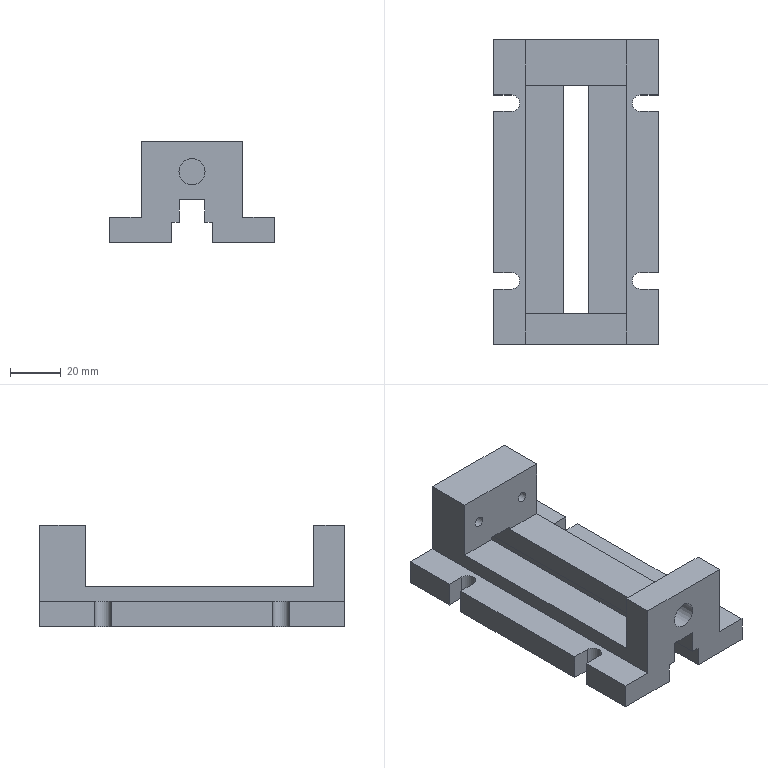Part | NX | features DATUM_CSYS 8, SKETCH 7, EXTRUDE 5, SIMPLE HOLE 5, HOLE PACKAGE 3, SYMBOLIC_THREAD 3 | 1 solid | 47 faces | box 65 x 120 x 40 mm | volume 106229 mm3 | plane 38 | cylinder 9 | commonest cylinder face diameters 6.5 x4 4.2 x2 5 x2 10.3 x1
STEP:
#1=CARTESIAN_POINT('',(-32.5,60.,0.));
#2=VERTEX_POINT('',#1);
#3=CARTESIAN_POINT('',(-32.5,38.25,0.));
#4=VERTEX_POINT('',#3);
#5=CARTESIAN_POINT('',(-32.5,60.,0.));
#6=DIRECTION('',(0.,-1.,0.));
#7=VECTOR('',#6,1000.);
#8=LINE('',#5,#7);
#9=EDGE_CURVE('',#2,#4,#8,.T.);
#10=ORIENTED_EDGE('',*,*,#9,.T.);
#11=CARTESIAN_POINT('',(-32.5,38.25,10.));
#12=VERTEX_POINT('',#11);
#13=CARTESIAN_POINT('',(-32.5,38.25,-1.));
#14=DIRECTION('',(0.,0.,-1.));
#15=VECTOR('',#14,1000.);
#16=LINE('',#13,#15);
#17=EDGE_CURVE('',#4,#12,#16,.F.);
#18=ORIENTED_EDGE('',*,*,#17,.T.);
#19=CARTESIAN_POINT('',(-32.5,60.,10.));
#20=VERTEX_POINT('',#19);
#21=CARTESIAN_POINT('',(-32.5,60.,10.));
#22=DIRECTION('',(0.,-1.,0.));
#23=VECTOR('',#22,1000.);
#24=LINE('',#21,#23);
#25=EDGE_CURVE('',#20,#12,#24,.T.);
#26=ORIENTED_EDGE('',*,*,#25,.F.);
#27=CARTESIAN_POINT('',(-32.5,60.,10.));
#28=DIRECTION('',(0.,0.,-1.));
#29=VECTOR('',#28,1000.);
#30=LINE('',#27,#29);
#31=EDGE_CURVE('',#20,#2,#30,.T.);
#32=ORIENTED_EDGE('',*,*,#31,.T.);
#33=EDGE_LOOP('',(#10,#18,#26,#32));
#34=FACE_BOUND('',#33,.T.);
#35=CARTESIAN_POINT('',(-32.5,60.,10.));
#36=DIRECTION('',(1.,0.,0.));
#37=DIRECTION('',(0.,1.,0.));
#38=AXIS2_PLACEMENT_3D('',#35,#36,#37);
#39=PLANE('',#38);
#40=ADVANCED_FACE('',(#34),#39,.F.);
#41=CARTESIAN_POINT('',(-32.5,31.75,10.));
#42=VERTEX_POINT('',#41);
#43=CARTESIAN_POINT('',(-32.5,-31.75,10.));
#44=VERTEX_POINT('',#43);
#45=CARTESIAN_POINT('',(-32.5,60.,10.));
#46=DIRECTION('',(0.,-1.,0.));
#47=VECTOR('',#46,1000.);
#48=LINE('',#45,#47);
#49=EDGE_CURVE('',#42,#44,#48,.T.);
#50=ORIENTED_EDGE('',*,*,#49,.F.);
#51=CARTESIAN_POINT('',(-32.5,31.75,0.));
#52=VERTEX_POINT('',#51);
#53=CARTESIAN_POINT('',(-32.5,31.75,-1.));
#54=DIRECTION('',(0.,0.,1.));
#55=VECTOR('',#54,1000.);
#56=LINE('',#53,#55);
#57=EDGE_CURVE('',#42,#52,#56,.F.);
#58=ORIENTED_EDGE('',*,*,#57,.T.);
#59=CARTESIAN_POINT('',(-32.5,-31.75,0.));
#60=VERTEX_POINT('',#59);
#61=CARTESIAN_POINT('',(-32.5,60.,0.));
#62=DIRECTION('',(0.,-1.,0.));
#63=VECTOR('',#62,1000.);
#64=LINE('',#61,#63);
#65=EDGE_CURVE('',#52,#60,#64,.T.);
#66=ORIENTED_EDGE('',*,*,#65,.T.);
#67=CARTESIAN_POINT('',(-32.5,-31.75,-1.));
#68=DIRECTION('',(0.,0.,-1.));
#69=VECTOR('',#68,1000.);
#70=LINE('',#67,#69);
#71=EDGE_CURVE('',#60,#44,#70,.F.);
#72=ORIENTED_EDGE('',*,*,#71,.T.);
#73=EDGE_LOOP('',(#50,#58,#66,#72));
#74=FACE_BOUND('',#73,.T.);
#75=CARTESIAN_POINT('',(-32.5,60.,10.));
#76=DIRECTION('',(1.,0.,0.));
#77=DIRECTION('',(0.,1.,0.));
#78=AXIS2_PLACEMENT_3D('',#75,#76,#77);
#79=PLANE('',#78);
#80=ADVANCED_FACE('',(#74),#79,.F.);
#81=CARTESIAN_POINT('',(32.5,-60.,0.));
#82=VERTEX_POINT('',#81);
#83=CARTESIAN_POINT('',(32.5,-38.25,0.));
#84=VERTEX_POINT('',#83);
#85=CARTESIAN_POINT('',(32.5,-60.,0.));
#86=DIRECTION('',(0.,1.,0.));
#87=VECTOR('',#86,1000.);
#88=LINE('',#85,#87);
#89=EDGE_CURVE('',#82,#84,#88,.T.);
#90=ORIENTED_EDGE('',*,*,#89,.T.);
#91=CARTESIAN_POINT('',(32.5,-38.25,10.));
#92=VERTEX_POINT('',#91);
#93=CARTESIAN_POINT('',(32.5,-38.25,-1.));
#94=DIRECTION('',(0.,0.,-1.));
#95=VECTOR('',#94,1000.);
#96=LINE('',#93,#95);
#97=EDGE_CURVE('',#84,#92,#96,.F.);
#98=ORIENTED_EDGE('',*,*,#97,.T.);
#99=CARTESIAN_POINT('',(32.5,-60.,10.));
#100=VERTEX_POINT('',#99);
#101=CARTESIAN_POINT('',(32.5,-60.,10.));
#102=DIRECTION('',(0.,1.,0.));
#103=VECTOR('',#102,1000.);
#104=LINE('',#101,#103);
#105=EDGE_CURVE('',#100,#92,#104,.T.);
#106=ORIENTED_EDGE('',*,*,#105,.F.);
#107=CARTESIAN_POINT('',(32.5,-60.,10.));
#108=DIRECTION('',(0.,0.,-1.));
#109=VECTOR('',#108,1000.);
#110=LINE('',#107,#109);
#111=EDGE_CURVE('',#100,#82,#110,.T.);
#112=ORIENTED_EDGE('',*,*,#111,.T.);
#113=EDGE_LOOP('',(#90,#98,#106,#112));
#114=FACE_BOUND('',#113,.T.);
#115=CARTESIAN_POINT('',(32.5,-60.,10.));
#116=DIRECTION('',(-1.,0.,0.));
#117=DIRECTION('',(0.,-1.,0.));
#118=AXIS2_PLACEMENT_3D('',#115,#116,#117);
#119=PLANE('',#118);
#120=ADVANCED_FACE('',(#114),#119,.F.);
#121=CARTESIAN_POINT('',(32.5,-31.75,10.));
#122=VERTEX_POINT('',#121);
#123=CARTESIAN_POINT('',(32.5,31.75,10.));
#124=VERTEX_POINT('',#123);
#125=CARTESIAN_POINT('',(32.5,-60.,10.));
#126=DIRECTION('',(0.,1.,0.));
#127=VECTOR('',#126,1000.);
#128=LINE('',#125,#127);
#129=EDGE_CURVE('',#122,#124,#128,.T.);
#130=ORIENTED_EDGE('',*,*,#129,.F.);
#131=CARTESIAN_POINT('',(32.5,-31.75,0.));
#132=VERTEX_POINT('',#131);
#133=CARTESIAN_POINT('',(32.5,-31.75,-1.));
#134=DIRECTION('',(0.,0.,1.));
#135=VECTOR('',#134,1000.);
#136=LINE('',#133,#135);
#137=EDGE_CURVE('',#122,#132,#136,.F.);
#138=ORIENTED_EDGE('',*,*,#137,.T.);
#139=CARTESIAN_POINT('',(32.5,31.75,0.));
#140=VERTEX_POINT('',#139);
#141=CARTESIAN_POINT('',(32.5,-60.,0.));
#142=DIRECTION('',(0.,1.,0.));
#143=VECTOR('',#142,1000.);
#144=LINE('',#141,#143);
#145=EDGE_CURVE('',#132,#140,#144,.T.);
#146=ORIENTED_EDGE('',*,*,#145,.T.);
#147=CARTESIAN_POINT('',(32.5,31.75,-1.));
#148=DIRECTION('',(0.,0.,-1.));
#149=VECTOR('',#148,1000.);
#150=LINE('',#147,#149);
#151=EDGE_CURVE('',#140,#124,#150,.F.);
#152=ORIENTED_EDGE('',*,*,#151,.T.);
#153=EDGE_LOOP('',(#130,#138,#146,#152));
#154=FACE_BOUND('',#153,.T.);
#155=CARTESIAN_POINT('',(32.5,-60.,10.));
#156=DIRECTION('',(-1.,0.,0.));
#157=DIRECTION('',(0.,-1.,0.));
#158=AXIS2_PLACEMENT_3D('',#155,#156,#157);
#159=PLANE('',#158);
#160=ADVANCED_FACE('',(#154),#159,.F.);
#161=ORIENTED_EDGE('',*,*,#25,.T.);
#162=CARTESIAN_POINT('',(-25.45,38.25,10.));
#163=VERTEX_POINT('',#162);
#164=CARTESIAN_POINT('',(-25.45,38.25,10.));
#165=DIRECTION('',(-1.,0.,0.));
#166=VECTOR('',#165,1000.);
#167=LINE('',#164,#166);
#168=EDGE_CURVE('',#12,#163,#167,.F.);
#169=ORIENTED_EDGE('',*,*,#168,.T.);
#170=CARTESIAN_POINT('',(-25.45,31.75,10.));
#171=VERTEX_POINT('',#170);
#172=CARTESIAN_POINT('',(-25.45,35.,10.));
#173=DIRECTION('',(0.,0.,1.));
#174=DIRECTION('',(0.,1.,0.));
#175=AXIS2_PLACEMENT_3D('',#172,#173,#174);
#176=CIRCLE('',#175,3.25);
#177=EDGE_CURVE('',#163,#171,#176,.F.);
#178=ORIENTED_EDGE('',*,*,#177,.T.);
#179=CARTESIAN_POINT('',(-32.5,31.75,10.));
#180=DIRECTION('',(1.,0.,0.));
#181=VECTOR('',#180,1000.);
#182=LINE('',#179,#181);
#183=EDGE_CURVE('',#171,#42,#182,.F.);
#184=ORIENTED_EDGE('',*,*,#183,.T.);
#185=ORIENTED_EDGE('',*,*,#49,.T.);
#186=CARTESIAN_POINT('',(-25.45,-31.75,10.));
#187=VERTEX_POINT('',#186);
#188=CARTESIAN_POINT('',(-25.45,-31.75,10.));
#189=DIRECTION('',(-1.,0.,0.));
#190=VECTOR('',#189,1000.);
#191=LINE('',#188,#190);
#192=EDGE_CURVE('',#44,#187,#191,.F.);
#193=ORIENTED_EDGE('',*,*,#192,.T.);
#194=CARTESIAN_POINT('',(-25.45,-38.25,10.));
#195=VERTEX_POINT('',#194);
#196=CARTESIAN_POINT('',(-25.45,-35.,10.));
#197=DIRECTION('',(0.,0.,1.));
#198=DIRECTION('',(0.,1.,0.));
#199=AXIS2_PLACEMENT_3D('',#196,#197,#198);
#200=CIRCLE('',#199,3.25);
#201=EDGE_CURVE('',#187,#195,#200,.F.);
#202=ORIENTED_EDGE('',*,*,#201,.T.);
#203=CARTESIAN_POINT('',(-32.5,-38.25,10.));
#204=VERTEX_POINT('',#203);
#205=CARTESIAN_POINT('',(-32.5,-38.25,10.));
#206=DIRECTION('',(1.,0.,0.));
#207=VECTOR('',#206,1000.);
#208=LINE('',#205,#207);
#209=EDGE_CURVE('',#195,#204,#208,.F.);
#210=ORIENTED_EDGE('',*,*,#209,.T.);
#211=CARTESIAN_POINT('',(-32.5,-60.,10.));
#212=VERTEX_POINT('',#211);
#213=CARTESIAN_POINT('',(-32.5,60.,10.));
#214=DIRECTION('',(0.,-1.,0.));
#215=VECTOR('',#214,1000.);
#216=LINE('',#213,#215);
#217=EDGE_CURVE('',#204,#212,#216,.T.);
#218=ORIENTED_EDGE('',*,*,#217,.T.);
#219=CARTESIAN_POINT('',(-20.,-60.,10.));
#220=VERTEX_POINT('',#219);
#221=CARTESIAN_POINT('',(-32.5,-60.,10.));
#222=DIRECTION('',(1.,0.,0.));
#223=VECTOR('',#222,1000.);
#224=LINE('',#221,#223);
#225=EDGE_CURVE('',#212,#220,#224,.T.);
#226=ORIENTED_EDGE('',*,*,#225,.T.);
#227=CARTESIAN_POINT('',(-20.,60.,10.));
#228=VERTEX_POINT('',#227);
#229=CARTESIAN_POINT('',(-20.,60.,10.));
#230=DIRECTION('',(0.,-1.,0.));
#231=VECTOR('',#230,1000.);
#232=LINE('',#229,#231);
#233=EDGE_CURVE('',#228,#220,#232,.T.);
#234=ORIENTED_EDGE('',*,*,#233,.F.);
#235=CARTESIAN_POINT('',(32.5,60.,10.));
#236=DIRECTION('',(-1.,0.,0.));
#237=VECTOR('',#236,1000.);
#238=LINE('',#235,#237);
#239=EDGE_CURVE('',#228,#20,#238,.T.);
#240=ORIENTED_EDGE('',*,*,#239,.T.);
#241=EDGE_LOOP('',(#161,#169,#178,#184,#185,#193,#202,#210,#218,#226,#234,#240));
#242=FACE_BOUND('',#241,.T.);
#243=CARTESIAN_POINT('',(0.,0.,10.));
#244=DIRECTION('',(0.,0.,1.));
#245=DIRECTION('',(1.,0.,0.));
#246=AXIS2_PLACEMENT_3D('',#243,#244,#245);
#247=PLANE('',#246);
#248=ADVANCED_FACE('',(#242),#247,.T.);
#249=CARTESIAN_POINT('',(25.45,-38.25,10.));
#250=VERTEX_POINT('',#249);
#251=CARTESIAN_POINT('',(25.45,-31.75,10.));
#252=VERTEX_POINT('',#251);
#253=CARTESIAN_POINT('',(25.45,-35.,10.));
#254=DIRECTION('',(0.,0.,1.));
#255=DIRECTION('',(0.,1.,0.));
#256=AXIS2_PLACEMENT_3D('',#253,#254,#255);
#257=CIRCLE('',#256,3.25);
#258=EDGE_CURVE('',#250,#252,#257,.F.);
#259=ORIENTED_EDGE('',*,*,#258,.T.);
#260=CARTESIAN_POINT('',(32.5,-31.75,10.));
#261=DIRECTION('',(-1.,0.,0.));
#262=VECTOR('',#261,1000.);
#263=LINE('',#260,#262);
#264=EDGE_CURVE('',#252,#122,#263,.F.);
#265=ORIENTED_EDGE('',*,*,#264,.T.);
#266=ORIENTED_EDGE('',*,*,#129,.T.);
#267=CARTESIAN_POINT('',(25.45,31.75,10.));
#268=VERTEX_POINT('',#267);
#269=CARTESIAN_POINT('',(25.45,31.75,10.));
#270=DIRECTION('',(1.,0.,0.));
#271=VECTOR('',#270,1000.);
#272=LINE('',#269,#271);
#273=EDGE_CURVE('',#124,#268,#272,.F.);
#274=ORIENTED_EDGE('',*,*,#273,.T.);
#275=CARTESIAN_POINT('',(25.45,38.25,10.));
#276=VERTEX_POINT('',#275);
#277=CARTESIAN_POINT('',(25.45,35.,10.));
#278=DIRECTION('',(0.,0.,1.));
#279=DIRECTION('',(0.,1.,0.));
#280=AXIS2_PLACEMENT_3D('',#277,#278,#279);
#281=CIRCLE('',#280,3.25);
#282=EDGE_CURVE('',#268,#276,#281,.F.);
#283=ORIENTED_EDGE('',*,*,#282,.T.);
#284=CARTESIAN_POINT('',(32.5,38.25,10.));
#285=VERTEX_POINT('',#284);
#286=CARTESIAN_POINT('',(32.5,38.25,10.));
#287=DIRECTION('',(-1.,0.,0.));
#288=VECTOR('',#287,1000.);
#289=LINE('',#286,#288);
#290=EDGE_CURVE('',#276,#285,#289,.F.);
#291=ORIENTED_EDGE('',*,*,#290,.T.);
#292=CARTESIAN_POINT('',(32.5,60.,10.));
#293=VERTEX_POINT('',#292);
#294=CARTESIAN_POINT('',(32.5,-60.,10.));
#295=DIRECTION('',(0.,1.,0.));
#296=VECTOR('',#295,1000.);
#297=LINE('',#294,#296);
#298=EDGE_CURVE('',#285,#293,#297,.T.);
#299=ORIENTED_EDGE('',*,*,#298,.T.);
#300=CARTESIAN_POINT('',(20.,60.,10.));
#301=VERTEX_POINT('',#300);
#302=CARTESIAN_POINT('',(32.5,60.,10.));
#303=DIRECTION('',(-1.,0.,0.));
#304=VECTOR('',#303,1000.);
#305=LINE('',#302,#304);
#306=EDGE_CURVE('',#293,#301,#305,.T.);
#307=ORIENTED_EDGE('',*,*,#306,.T.);
#308=CARTESIAN_POINT('',(20.,-60.,10.));
#309=VERTEX_POINT('',#308);
#310=CARTESIAN_POINT('',(20.,-60.,10.));
#311=DIRECTION('',(0.,1.,0.));
#312=VECTOR('',#311,1000.);
#313=LINE('',#310,#312);
#314=EDGE_CURVE('',#309,#301,#313,.T.);
#315=ORIENTED_EDGE('',*,*,#314,.F.);
#316=CARTESIAN_POINT('',(-32.5,-60.,10.));
#317=DIRECTION('',(1.,0.,0.));
#318=VECTOR('',#317,1000.);
#319=LINE('',#316,#318);
#320=EDGE_CURVE('',#309,#100,#319,.T.);
#321=ORIENTED_EDGE('',*,*,#320,.T.);
#322=ORIENTED_EDGE('',*,*,#105,.T.);
#323=CARTESIAN_POINT('',(25.45,-38.25,10.));
#324=DIRECTION('',(1.,0.,0.));
#325=VECTOR('',#324,1000.);
#326=LINE('',#323,#325);
#327=EDGE_CURVE('',#92,#250,#326,.F.);
#328=ORIENTED_EDGE('',*,*,#327,.T.);
#329=EDGE_LOOP('',(#259,#265,#266,#274,#283,#291,#299,#307,#315,#321,#322,#328));
#330=FACE_BOUND('',#329,.T.);
#331=CARTESIAN_POINT('',(0.,0.,10.));
#332=DIRECTION('',(0.,0.,1.));
#333=DIRECTION('',(1.,0.,0.));
#334=AXIS2_PLACEMENT_3D('',#331,#332,#333);
#335=PLANE('',#334);
#336=ADVANCED_FACE('',(#330),#335,.T.);
#337=ORIENTED_EDGE('',*,*,#65,.F.);
#338=CARTESIAN_POINT('',(-25.45,31.75,0.));
#339=VERTEX_POINT('',#338);
#340=CARTESIAN_POINT('',(-32.5,31.75,0.));
#341=DIRECTION('',(-1.,0.,0.));
#342=VECTOR('',#341,1000.);
#343=LINE('',#340,#342);
#344=EDGE_CURVE('',#52,#339,#343,.F.);
#345=ORIENTED_EDGE('',*,*,#344,.T.);
#346=CARTESIAN_POINT('',(-25.45,38.25,0.));
#347=VERTEX_POINT('',#346);
#348=CARTESIAN_POINT('',(-25.45,35.,0.));
#349=DIRECTION('',(0.,0.,1.));
#350=DIRECTION('',(1.,0.,0.));
#351=AXIS2_PLACEMENT_3D('',#348,#349,#350);
#352=CIRCLE('',#351,3.25);
#353=EDGE_CURVE('',#339,#347,#352,.T.);
#354=ORIENTED_EDGE('',*,*,#353,.T.);
#355=CARTESIAN_POINT('',(-25.45,38.25,0.));
#356=DIRECTION('',(1.,0.,0.));
#357=VECTOR('',#356,1000.);
#358=LINE('',#355,#357);
#359=EDGE_CURVE('',#347,#4,#358,.F.);
#360=ORIENTED_EDGE('',*,*,#359,.T.);
#361=ORIENTED_EDGE('',*,*,#9,.F.);
#362=CARTESIAN_POINT('',(-8.,60.,0.));
#363=VERTEX_POINT('',#362);
#364=CARTESIAN_POINT('',(32.5,60.,0.));
#365=DIRECTION('',(-1.,0.,0.));
#366=VECTOR('',#365,1000.);
#367=LINE('',#364,#366);
#368=EDGE_CURVE('',#363,#2,#367,.T.);
#369=ORIENTED_EDGE('',*,*,#368,.F.);
#370=CARTESIAN_POINT('',(-8.,-60.,0.));
#371=VERTEX_POINT('',#370);
#372=CARTESIAN_POINT('',(-8.,54940.,0.));
#373=DIRECTION('',(0.,1.,0.));
#374=VECTOR('',#373,1000.);
#375=LINE('',#372,#374);
#376=EDGE_CURVE('',#363,#371,#375,.F.);
#377=ORIENTED_EDGE('',*,*,#376,.T.);
#378=CARTESIAN_POINT('',(-32.5,-60.,0.));
#379=VERTEX_POINT('',#378);
#380=CARTESIAN_POINT('',(-32.5,-60.,0.));
#381=DIRECTION('',(1.,0.,0.));
#382=VECTOR('',#381,1000.);
#383=LINE('',#380,#382);
#384=EDGE_CURVE('',#379,#371,#383,.T.);
#385=ORIENTED_EDGE('',*,*,#384,.F.);
#386=CARTESIAN_POINT('',(-32.5,-38.25,0.));
#387=VERTEX_POINT('',#386);
#388=CARTESIAN_POINT('',(-32.5,60.,0.));
#389=DIRECTION('',(0.,-1.,0.));
#390=VECTOR('',#389,1000.);
#391=LINE('',#388,#390);
#392=EDGE_CURVE('',#387,#379,#391,.T.);
#393=ORIENTED_EDGE('',*,*,#392,.F.);
#394=CARTESIAN_POINT('',(-25.45,-38.25,0.));
#395=VERTEX_POINT('',#394);
#396=CARTESIAN_POINT('',(-32.5,-38.25,0.));
#397=DIRECTION('',(-1.,0.,0.));
#398=VECTOR('',#397,1000.);
#399=LINE('',#396,#398);
#400=EDGE_CURVE('',#387,#395,#399,.F.);
#401=ORIENTED_EDGE('',*,*,#400,.T.);
#402=CARTESIAN_POINT('',(-25.45,-31.75,0.));
#403=VERTEX_POINT('',#402);
#404=CARTESIAN_POINT('',(-25.45,-35.,0.));
#405=DIRECTION('',(0.,0.,1.));
#406=DIRECTION('',(1.,0.,0.));
#407=AXIS2_PLACEMENT_3D('',#404,#405,#406);
#408=CIRCLE('',#407,3.25);
#409=EDGE_CURVE('',#395,#403,#408,.T.);
#410=ORIENTED_EDGE('',*,*,#409,.T.);
#411=CARTESIAN_POINT('',(-25.45,-31.75,0.));
#412=DIRECTION('',(1.,0.,0.));
#413=VECTOR('',#412,1000.);
#414=LINE('',#411,#413);
#415=EDGE_CURVE('',#403,#60,#414,.F.);
#416=ORIENTED_EDGE('',*,*,#415,.T.);
#417=EDGE_LOOP('',(#337,#345,#354,#360,#361,#369,#377,#385,#393,#401,#410,#416));
#418=FACE_BOUND('',#417,.T.);
#419=CARTESIAN_POINT('',(0.,0.,0.));
#420=DIRECTION('',(0.,0.,1.));
#421=DIRECTION('',(1.,0.,0.));
#422=AXIS2_PLACEMENT_3D('',#419,#420,#421);
#423=PLANE('',#422);
#424=ADVANCED_FACE('',(#418),#423,.F.);
#425=CARTESIAN_POINT('',(5.,42.,16.));
#426=VERTEX_POINT('',#425);
#427=CARTESIAN_POINT('',(5.,-48.,16.));
#428=VERTEX_POINT('',#427);
#429=CARTESIAN_POINT('',(5.,54940.,16.));
#430=DIRECTION('',(0.,-1.,0.));
#431=VECTOR('',#430,1000.);
#432=LINE('',#429,#431);
#433=EDGE_CURVE('',#426,#428,#432,.T.);
#434=ORIENTED_EDGE('',*,*,#433,.T.);
#435=CARTESIAN_POINT('',(20.,-48.,16.));
#436=VERTEX_POINT('',#435);
#437=CARTESIAN_POINT('',(-20.,-48.,16.));
#438=DIRECTION('',(1.,0.,0.));
#439=VECTOR('',#438,1000.);
#440=LINE('',#437,#439);
#441=EDGE_CURVE('',#436,#428,#440,.F.);
#442=ORIENTED_EDGE('',*,*,#441,.F.);
#443=CARTESIAN_POINT('',(20.,42.,16.));
#444=VERTEX_POINT('',#443);
#445=CARTESIAN_POINT('',(20.,-48.,16.));
#446=DIRECTION('',(0.,1.,0.));
#447=VECTOR('',#446,1000.);
#448=LINE('',#445,#447);
#449=EDGE_CURVE('',#436,#444,#448,.T.);
#450=ORIENTED_EDGE('',*,*,#449,.T.);
#451=CARTESIAN_POINT('',(20.,42.,16.));
#452=DIRECTION('',(-1.,0.,0.));
#453=VECTOR('',#452,1000.);
#454=LINE('',#451,#453);
#455=EDGE_CURVE('',#426,#444,#454,.F.);
#456=ORIENTED_EDGE('',*,*,#455,.F.);
#457=EDGE_LOOP('',(#434,#442,#450,#456));
#458=FACE_BOUND('',#457,.T.);
#459=CARTESIAN_POINT('',(0.,0.,16.));
#460=DIRECTION('',(0.,0.,1.));
#461=DIRECTION('',(1.,0.,0.));
#462=AXIS2_PLACEMENT_3D('',#459,#460,#461);
#463=PLANE('',#462);
#464=ADVANCED_FACE('',(#458),#463,.T.);
#465=CARTESIAN_POINT('',(-20.,-48.,40.));
#466=VERTEX_POINT('',#465);
#467=CARTESIAN_POINT('',(20.,-48.,40.));
#468=VERTEX_POINT('',#467);
#469=CARTESIAN_POINT('',(-20.,-48.,40.));
#470=DIRECTION('',(1.,0.,0.));
#471=VECTOR('',#470,1000.);
#472=LINE('',#469,#471);
#473=EDGE_CURVE('',#466,#468,#472,.T.);
#474=ORIENTED_EDGE('',*,*,#473,.F.);
#475=CARTESIAN_POINT('',(-20.,-60.,40.));
#476=VERTEX_POINT('',#475);
#477=CARTESIAN_POINT('',(-20.,60.,40.));
#478=DIRECTION('',(0.,-1.,0.));
#479=VECTOR('',#478,1000.);
#480=LINE('',#477,#479);
#481=EDGE_CURVE('',#466,#476,#480,.T.);
#482=ORIENTED_EDGE('',*,*,#481,.T.);
#483=CARTESIAN_POINT('',(20.,-60.,40.));
#484=VERTEX_POINT('',#483);
#485=CARTESIAN_POINT('',(-20.,-60.,40.));
#486=DIRECTION('',(1.,0.,0.));
#487=VECTOR('',#486,1000.);
#488=LINE('',#485,#487);
#489=EDGE_CURVE('',#476,#484,#488,.T.);
#490=ORIENTED_EDGE('',*,*,#489,.T.);
#491=CARTESIAN_POINT('',(20.,-60.,40.));
#492=DIRECTION('',(0.,1.,0.));
#493=VECTOR('',#492,1000.);
#494=LINE('',#491,#493);
#495=EDGE_CURVE('',#484,#468,#494,.T.);
#496=ORIENTED_EDGE('',*,*,#495,.T.);
#497=EDGE_LOOP('',(#474,#482,#490,#496));
#498=FACE_BOUND('',#497,.T.);
#499=CARTESIAN_POINT('',(0.,0.,40.));
#500=DIRECTION('',(0.,0.,1.));
#501=DIRECTION('',(1.,0.,0.));
#502=AXIS2_PLACEMENT_3D('',#499,#500,#501);
#503=PLANE('',#502);
#504=ADVANCED_FACE('',(#498),#503,.T.);
#505=ORIENTED_EDGE('',*,*,#217,.F.);
#506=CARTESIAN_POINT('',(-32.5,-38.25,-1.));
#507=DIRECTION('',(0.,0.,1.));
#508=VECTOR('',#507,1000.);
#509=LINE('',#506,#508);
#510=EDGE_CURVE('',#204,#387,#509,.F.);
#511=ORIENTED_EDGE('',*,*,#510,.T.);
#512=ORIENTED_EDGE('',*,*,#392,.T.);
#513=CARTESIAN_POINT('',(-32.5,-60.,10.));
#514=DIRECTION('',(0.,0.,-1.));
#515=VECTOR('',#514,1000.);
#516=LINE('',#513,#515);
#517=EDGE_CURVE('',#212,#379,#516,.T.);
#518=ORIENTED_EDGE('',*,*,#517,.F.);
#519=EDGE_LOOP('',(#505,#511,#512,#518));
#520=FACE_BOUND('',#519,.T.);
#521=CARTESIAN_POINT('',(-32.5,60.,10.));
#522=DIRECTION('',(1.,0.,0.));
#523=DIRECTION('',(0.,1.,0.));
#524=AXIS2_PLACEMENT_3D('',#521,#522,#523);
#525=PLANE('',#524);
#526=ADVANCED_FACE('',(#520),#525,.F.);
#527=CARTESIAN_POINT('',(-5.15,-60.,28.));
#528=VERTEX_POINT('',#527);
#529=CARTESIAN_POINT('',(0.,-60.,28.));
#530=DIRECTION('',(0.,1.,0.));
#531=DIRECTION('',(-1.,0.,0.));
#532=AXIS2_PLACEMENT_3D('',#529,#530,#531);
#533=CIRCLE('',#532,5.15);
#534=EDGE_CURVE('',#528,#528,#533,.T.);
#535=ORIENTED_EDGE('',*,*,#534,.T.);
#536=EDGE_LOOP('',(#535));
#537=FACE_BOUND('',#536,.T.);
#538=ORIENTED_EDGE('',*,*,#384,.T.);
#539=CARTESIAN_POINT('',(-8.,-60.,8.));
#540=VERTEX_POINT('',#539);
#541=CARTESIAN_POINT('',(-8.,-60.,8.));
#542=DIRECTION('',(0.,0.,-1.));
#543=VECTOR('',#542,1000.);
#544=LINE('',#541,#543);
#545=EDGE_CURVE('',#371,#540,#544,.F.);
#546=ORIENTED_EDGE('',*,*,#545,.T.);
#547=CARTESIAN_POINT('',(-5.,-60.,8.));
#548=VERTEX_POINT('',#547);
#549=CARTESIAN_POINT('',(-5.,-60.,8.));
#550=DIRECTION('',(-1.,0.,0.));
#551=VECTOR('',#550,1000.);
#552=LINE('',#549,#551);
#553=EDGE_CURVE('',#540,#548,#552,.F.);
#554=ORIENTED_EDGE('',*,*,#553,.T.);
#555=CARTESIAN_POINT('',(-5.,-60.,17.));
#556=VERTEX_POINT('',#555);
#557=CARTESIAN_POINT('',(-5.,-60.,17.));
#558=DIRECTION('',(0.,0.,-1.));
#559=VECTOR('',#558,1000.);
#560=LINE('',#557,#559);
#561=EDGE_CURVE('',#548,#556,#560,.F.);
#562=ORIENTED_EDGE('',*,*,#561,.T.);
#563=CARTESIAN_POINT('',(5.,-60.,17.));
#564=VERTEX_POINT('',#563);
#565=CARTESIAN_POINT('',(5.,-60.,17.));
#566=DIRECTION('',(-1.,0.,0.));
#567=VECTOR('',#566,1000.);
#568=LINE('',#565,#567);
#569=EDGE_CURVE('',#556,#564,#568,.F.);
#570=ORIENTED_EDGE('',*,*,#569,.T.);
#571=CARTESIAN_POINT('',(5.,-60.,8.));
#572=VERTEX_POINT('',#571);
#573=CARTESIAN_POINT('',(5.,-60.,8.));
#574=DIRECTION('',(0.,0.,1.));
#575=VECTOR('',#574,1000.);
#576=LINE('',#573,#575);
#577=EDGE_CURVE('',#564,#572,#576,.F.);
#578=ORIENTED_EDGE('',*,*,#577,.T.);
#579=CARTESIAN_POINT('',(8.,-60.,8.));
#580=VERTEX_POINT('',#579);
#581=CARTESIAN_POINT('',(8.,-60.,8.));
#582=DIRECTION('',(-1.,0.,0.));
#583=VECTOR('',#582,1000.);
#584=LINE('',#581,#583);
#585=EDGE_CURVE('',#572,#580,#584,.F.);
#586=ORIENTED_EDGE('',*,*,#585,.T.);
#587=CARTESIAN_POINT('',(8.,-60.,0.));
#588=VERTEX_POINT('',#587);
#589=CARTESIAN_POINT('',(8.,-60.,0.));
#590=DIRECTION('',(0.,0.,1.));
#591=VECTOR('',#590,1000.);
#592=LINE('',#589,#591);
#593=EDGE_CURVE('',#580,#588,#592,.F.);
#594=ORIENTED_EDGE('',*,*,#593,.T.);
#595=CARTESIAN_POINT('',(-32.5,-60.,0.));
#596=DIRECTION('',(1.,0.,0.));
#597=VECTOR('',#596,1000.);
#598=LINE('',#595,#597);
#599=EDGE_CURVE('',#588,#82,#598,.T.);
#600=ORIENTED_EDGE('',*,*,#599,.T.);
#601=ORIENTED_EDGE('',*,*,#111,.F.);
#602=ORIENTED_EDGE('',*,*,#320,.F.);
#603=CARTESIAN_POINT('',(20.,-60.,40.));
#604=DIRECTION('',(0.,0.,-1.));
#605=VECTOR('',#604,1000.);
#606=LINE('',#603,#605);
#607=EDGE_CURVE('',#484,#309,#606,.T.);
#608=ORIENTED_EDGE('',*,*,#607,.F.);
#609=ORIENTED_EDGE('',*,*,#489,.F.);
#610=CARTESIAN_POINT('',(-20.,-60.,40.));
#611=DIRECTION('',(0.,0.,-1.));
#612=VECTOR('',#611,1000.);
#613=LINE('',#610,#612);
#614=EDGE_CURVE('',#476,#220,#613,.T.);
#615=ORIENTED_EDGE('',*,*,#614,.T.);
#616=ORIENTED_EDGE('',*,*,#225,.F.);
#617=ORIENTED_EDGE('',*,*,#517,.T.);
#618=EDGE_LOOP('',(#538,#546,#554,#562,#570,#578,#586,#594,#600,#601,#602,#608,#609,#615,#616,#617));
#619=FACE_BOUND('',#618,.T.);
#620=CARTESIAN_POINT('',(-32.5,-60.,10.));
#621=DIRECTION('',(0.,1.,0.));
#622=DIRECTION('',(-1.,0.,0.));
#623=AXIS2_PLACEMENT_3D('',#620,#621,#622);
#624=PLANE('',#623);
#625=ADVANCED_FACE('',(#537,#619),#624,.F.);
#626=ORIENTED_EDGE('',*,*,#298,.F.);
#627=CARTESIAN_POINT('',(32.5,38.25,0.));
#628=VERTEX_POINT('',#627);
#629=CARTESIAN_POINT('',(32.5,38.25,-1.));
#630=DIRECTION('',(0.,0.,1.));
#631=VECTOR('',#630,1000.);
#632=LINE('',#629,#631);
#633=EDGE_CURVE('',#285,#628,#632,.F.);
#634=ORIENTED_EDGE('',*,*,#633,.T.);
#635=CARTESIAN_POINT('',(32.5,60.,0.));
#636=VERTEX_POINT('',#635);
#637=CARTESIAN_POINT('',(32.5,-60.,0.));
#638=DIRECTION('',(0.,1.,0.));
#639=VECTOR('',#638,1000.);
#640=LINE('',#637,#639);
#641=EDGE_CURVE('',#628,#636,#640,.T.);
#642=ORIENTED_EDGE('',*,*,#641,.T.);
#643=CARTESIAN_POINT('',(32.5,60.,10.));
#644=DIRECTION('',(0.,0.,-1.));
#645=VECTOR('',#644,1000.);
#646=LINE('',#643,#645);
#647=EDGE_CURVE('',#293,#636,#646,.T.);
#648=ORIENTED_EDGE('',*,*,#647,.F.);
#649=EDGE_LOOP('',(#626,#634,#642,#648));
#650=FACE_BOUND('',#649,.T.);
#651=CARTESIAN_POINT('',(32.5,-60.,10.));
#652=DIRECTION('',(-1.,0.,0.));
#653=DIRECTION('',(0.,-1.,0.));
#654=AXIS2_PLACEMENT_3D('',#651,#652,#653);
#655=PLANE('',#654);
#656=ADVANCED_FACE('',(#650),#655,.F.);
#657=CARTESIAN_POINT('',(14.5,60.,28.));
#658=VERTEX_POINT('',#657);
#659=CARTESIAN_POINT('',(12.,60.,28.));
#660=DIRECTION('',(0.,-1.,0.));
#661=DIRECTION('',(1.,0.,0.));
#662=AXIS2_PLACEMENT_3D('',#659,#660,#661);
#663=CIRCLE('',#662,2.5);
#664=EDGE_CURVE('',#658,#658,#663,.T.);
#665=ORIENTED_EDGE('',*,*,#664,.T.);
#666=EDGE_LOOP('',(#665));
#667=FACE_BOUND('',#666,.T.);
#668=CARTESIAN_POINT('',(-9.5,60.,28.));
#669=VERTEX_POINT('',#668);
#670=CARTESIAN_POINT('',(-12.,60.,28.));
#671=DIRECTION('',(0.,-1.,0.));
#672=DIRECTION('',(1.,0.,0.));
#673=AXIS2_PLACEMENT_3D('',#670,#671,#672);
#674=CIRCLE('',#673,2.5);
#675=EDGE_CURVE('',#669,#669,#674,.T.);
#676=ORIENTED_EDGE('',*,*,#675,.T.);
#677=EDGE_LOOP('',(#676));
#678=FACE_BOUND('',#677,.T.);
#679=CARTESIAN_POINT('',(-5.,60.,8.));
#680=VERTEX_POINT('',#679);
#681=CARTESIAN_POINT('',(-8.,60.,8.));
#682=VERTEX_POINT('',#681);
#683=CARTESIAN_POINT('',(-5.,60.,8.));
#684=DIRECTION('',(1.,0.,0.));
#685=VECTOR('',#684,1000.);
#686=LINE('',#683,#685);
#687=EDGE_CURVE('',#680,#682,#686,.F.);
#688=ORIENTED_EDGE('',*,*,#687,.T.);
#689=CARTESIAN_POINT('',(-8.,60.,8.));
#690=DIRECTION('',(0.,0.,1.));
#691=VECTOR('',#690,1000.);
#692=LINE('',#689,#691);
#693=EDGE_CURVE('',#682,#363,#692,.F.);
#694=ORIENTED_EDGE('',*,*,#693,.T.);
#695=ORIENTED_EDGE('',*,*,#368,.T.);
#696=ORIENTED_EDGE('',*,*,#31,.F.);
#697=ORIENTED_EDGE('',*,*,#239,.F.);
#698=CARTESIAN_POINT('',(-20.,60.,40.));
#699=VERTEX_POINT('',#698);
#700=CARTESIAN_POINT('',(-20.,60.,40.));
#701=DIRECTION('',(0.,0.,-1.));
#702=VECTOR('',#701,1000.);
#703=LINE('',#700,#702);
#704=EDGE_CURVE('',#699,#228,#703,.T.);
#705=ORIENTED_EDGE('',*,*,#704,.F.);
#706=CARTESIAN_POINT('',(20.,60.,40.));
#707=VERTEX_POINT('',#706);
#708=CARTESIAN_POINT('',(20.,60.,40.));
#709=DIRECTION('',(-1.,0.,0.));
#710=VECTOR('',#709,1000.);
#711=LINE('',#708,#710);
#712=EDGE_CURVE('',#707,#699,#711,.T.);
#713=ORIENTED_EDGE('',*,*,#712,.F.);
#714=CARTESIAN_POINT('',(20.,60.,40.));
#715=DIRECTION('',(0.,0.,-1.));
#716=VECTOR('',#715,1000.);
#717=LINE('',#714,#716);
#718=EDGE_CURVE('',#707,#301,#717,.T.);
#719=ORIENTED_EDGE('',*,*,#718,.T.);
#720=ORIENTED_EDGE('',*,*,#306,.F.);
#721=ORIENTED_EDGE('',*,*,#647,.T.);
#722=CARTESIAN_POINT('',(8.,60.,0.));
#723=VERTEX_POINT('',#722);
#724=CARTESIAN_POINT('',(32.5,60.,0.));
#725=DIRECTION('',(-1.,0.,0.));
#726=VECTOR('',#725,1000.);
#727=LINE('',#724,#726);
#728=EDGE_CURVE('',#636,#723,#727,.T.);
#729=ORIENTED_EDGE('',*,*,#728,.T.);
#730=CARTESIAN_POINT('',(8.,60.,8.));
#731=VERTEX_POINT('',#730);
#732=CARTESIAN_POINT('',(8.,60.,0.));
#733=DIRECTION('',(0.,0.,-1.));
#734=VECTOR('',#733,1000.);
#735=LINE('',#732,#734);
#736=EDGE_CURVE('',#723,#731,#735,.F.);
#737=ORIENTED_EDGE('',*,*,#736,.T.);
#738=CARTESIAN_POINT('',(5.,60.,8.));
#739=VERTEX_POINT('',#738);
#740=CARTESIAN_POINT('',(8.,60.,8.));
#741=DIRECTION('',(1.,0.,0.));
#742=VECTOR('',#741,1000.);
#743=LINE('',#740,#742);
#744=EDGE_CURVE('',#731,#739,#743,.F.);
#745=ORIENTED_EDGE('',*,*,#744,.T.);
#746=CARTESIAN_POINT('',(5.,60.,17.));
#747=VERTEX_POINT('',#746);
#748=CARTESIAN_POINT('',(5.,60.,8.));
#749=DIRECTION('',(0.,0.,-1.));
#750=VECTOR('',#749,1000.);
#751=LINE('',#748,#750);
#752=EDGE_CURVE('',#739,#747,#751,.F.);
#753=ORIENTED_EDGE('',*,*,#752,.T.);
#754=CARTESIAN_POINT('',(-5.,60.,17.));
#755=VERTEX_POINT('',#754);
#756=CARTESIAN_POINT('',(5.,60.,17.));
#757=DIRECTION('',(1.,0.,0.));
#758=VECTOR('',#757,1000.);
#759=LINE('',#756,#758);
#760=EDGE_CURVE('',#747,#755,#759,.F.);
#761=ORIENTED_EDGE('',*,*,#760,.T.);
#762=CARTESIAN_POINT('',(-5.,60.,17.));
#763=DIRECTION('',(0.,0.,1.));
#764=VECTOR('',#763,1000.);
#765=LINE('',#762,#764);
#766=EDGE_CURVE('',#755,#680,#765,.F.);
#767=ORIENTED_EDGE('',*,*,#766,.T.);
#768=EDGE_LOOP('',(#688,#694,#695,#696,#697,#705,#713,#719,#720,#721,#729,#737,#745,#753,#761,#767));
#769=FACE_BOUND('',#768,.T.);
#770=CARTESIAN_POINT('',(32.5,60.,10.));
#771=DIRECTION('',(0.,-1.,0.));
#772=DIRECTION('',(1.,0.,0.));
#773=AXIS2_PLACEMENT_3D('',#770,#771,#772);
#774=PLANE('',#773);
#775=ADVANCED_FACE('',(#667,#678,#769),#774,.F.);
#776=ORIENTED_EDGE('',*,*,#145,.F.);
#777=CARTESIAN_POINT('',(25.45,-31.75,0.));
#778=VERTEX_POINT('',#777);
#779=CARTESIAN_POINT('',(32.5,-31.75,0.));
#780=DIRECTION('',(1.,0.,0.));
#781=VECTOR('',#780,1000.);
#782=LINE('',#779,#781);
#783=EDGE_CURVE('',#132,#778,#782,.F.);
#784=ORIENTED_EDGE('',*,*,#783,.T.);
#785=CARTESIAN_POINT('',(25.45,-38.25,0.));
#786=VERTEX_POINT('',#785);
#787=CARTESIAN_POINT('',(25.45,-35.,0.));
#788=DIRECTION('',(0.,0.,1.));
#789=DIRECTION('',(1.,0.,0.));
#790=AXIS2_PLACEMENT_3D('',#787,#788,#789);
#791=CIRCLE('',#790,3.25);
#792=EDGE_CURVE('',#778,#786,#791,.T.);
#793=ORIENTED_EDGE('',*,*,#792,.T.);
#794=CARTESIAN_POINT('',(25.45,-38.25,0.));
#795=DIRECTION('',(-1.,0.,0.));
#796=VECTOR('',#795,1000.);
#797=LINE('',#794,#796);
#798=EDGE_CURVE('',#786,#84,#797,.F.);
#799=ORIENTED_EDGE('',*,*,#798,.T.);
#800=ORIENTED_EDGE('',*,*,#89,.F.);
#801=ORIENTED_EDGE('',*,*,#599,.F.);
#802=CARTESIAN_POINT('',(8.,54940.,0.));
#803=DIRECTION('',(0.,-1.,0.));
#804=VECTOR('',#803,1000.);
#805=LINE('',#802,#804);
#806=EDGE_CURVE('',#588,#723,#805,.F.);
#807=ORIENTED_EDGE('',*,*,#806,.T.);
#808=ORIENTED_EDGE('',*,*,#728,.F.);
#809=ORIENTED_EDGE('',*,*,#641,.F.);
#810=CARTESIAN_POINT('',(25.45,38.25,0.));
#811=VERTEX_POINT('',#810);
#812=CARTESIAN_POINT('',(32.5,38.25,0.));
#813=DIRECTION('',(1.,0.,0.));
#814=VECTOR('',#813,1000.);
#815=LINE('',#812,#814);
#816=EDGE_CURVE('',#628,#811,#815,.F.);
#817=ORIENTED_EDGE('',*,*,#816,.T.);
#818=CARTESIAN_POINT('',(25.45,31.75,0.));
#819=VERTEX_POINT('',#818);
#820=CARTESIAN_POINT('',(25.45,35.,0.));
#821=DIRECTION('',(0.,0.,1.));
#822=DIRECTION('',(1.,0.,0.));
#823=AXIS2_PLACEMENT_3D('',#820,#821,#822);
#824=CIRCLE('',#823,3.25);
#825=EDGE_CURVE('',#811,#819,#824,.T.);
#826=ORIENTED_EDGE('',*,*,#825,.T.);
#827=CARTESIAN_POINT('',(25.45,31.75,0.));
#828=DIRECTION('',(-1.,0.,0.));
#829=VECTOR('',#828,1000.);
#830=LINE('',#827,#829);
#831=EDGE_CURVE('',#819,#140,#830,.F.);
#832=ORIENTED_EDGE('',*,*,#831,.T.);
#833=EDGE_LOOP('',(#776,#784,#793,#799,#800,#801,#807,#808,#809,#817,#826,#832));
#834=FACE_BOUND('',#833,.T.);
#835=CARTESIAN_POINT('',(0.,0.,0.));
#836=DIRECTION('',(0.,0.,1.));
#837=DIRECTION('',(1.,0.,0.));
#838=AXIS2_PLACEMENT_3D('',#835,#836,#837);
#839=PLANE('',#838);
#840=ADVANCED_FACE('',(#834),#839,.F.);
#841=CARTESIAN_POINT('',(-20.,42.,16.));
#842=VERTEX_POINT('',#841);
#843=CARTESIAN_POINT('',(-20.,-48.,16.));
#844=VERTEX_POINT('',#843);
#845=CARTESIAN_POINT('',(-20.,42.,16.));
#846=DIRECTION('',(0.,-1.,0.));
#847=VECTOR('',#846,1000.);
#848=LINE('',#845,#847);
#849=EDGE_CURVE('',#842,#844,#848,.T.);
#850=ORIENTED_EDGE('',*,*,#849,.F.);
#851=CARTESIAN_POINT('',(-20.,42.,40.));
#852=VERTEX_POINT('',#851);
#853=CARTESIAN_POINT('',(-20.,42.,16.));
#854=DIRECTION('',(0.,0.,1.));
#855=VECTOR('',#854,1000.);
#856=LINE('',#853,#855);
#857=EDGE_CURVE('',#842,#852,#856,.T.);
#858=ORIENTED_EDGE('',*,*,#857,.T.);
#859=CARTESIAN_POINT('',(-20.,60.,40.));
#860=DIRECTION('',(0.,-1.,0.));
#861=VECTOR('',#860,1000.);
#862=LINE('',#859,#861);
#863=EDGE_CURVE('',#699,#852,#862,.T.);
#864=ORIENTED_EDGE('',*,*,#863,.F.);
#865=ORIENTED_EDGE('',*,*,#704,.T.);
#866=ORIENTED_EDGE('',*,*,#233,.T.);
#867=ORIENTED_EDGE('',*,*,#614,.F.);
#868=ORIENTED_EDGE('',*,*,#481,.F.);
#869=CARTESIAN_POINT('',(-20.,-48.,16.));
#870=DIRECTION('',(0.,0.,1.));
#871=VECTOR('',#870,1000.);
#872=LINE('',#869,#871);
#873=EDGE_CURVE('',#844,#466,#872,.T.);
#874=ORIENTED_EDGE('',*,*,#873,.F.);
#875=EDGE_LOOP('',(#850,#858,#864,#865,#866,#867,#868,#874));
#876=FACE_BOUND('',#875,.T.);
#877=CARTESIAN_POINT('',(-20.,60.,40.));
#878=DIRECTION('',(1.,0.,0.));
#879=DIRECTION('',(0.,1.,0.));
#880=AXIS2_PLACEMENT_3D('',#877,#878,#879);
#881=PLANE('',#880);
#882=ADVANCED_FACE('',(#876),#881,.F.);
#883=ORIENTED_EDGE('',*,*,#449,.F.);
#884=CARTESIAN_POINT('',(20.,-48.,16.));
#885=DIRECTION('',(0.,0.,1.));
#886=VECTOR('',#885,1000.);
#887=LINE('',#884,#886);
#888=EDGE_CURVE('',#436,#468,#887,.T.);
#889=ORIENTED_EDGE('',*,*,#888,.T.);
#890=ORIENTED_EDGE('',*,*,#495,.F.);
#891=ORIENTED_EDGE('',*,*,#607,.T.);
#892=ORIENTED_EDGE('',*,*,#314,.T.);
#893=ORIENTED_EDGE('',*,*,#718,.F.);
#894=CARTESIAN_POINT('',(20.,42.,40.));
#895=VERTEX_POINT('',#894);
#896=CARTESIAN_POINT('',(20.,-60.,40.));
#897=DIRECTION('',(0.,1.,0.));
#898=VECTOR('',#897,1000.);
#899=LINE('',#896,#898);
#900=EDGE_CURVE('',#895,#707,#899,.T.);
#901=ORIENTED_EDGE('',*,*,#900,.F.);
#902=CARTESIAN_POINT('',(20.,42.,16.));
#903=DIRECTION('',(0.,0.,1.));
#904=VECTOR('',#903,1000.);
#905=LINE('',#902,#904);
#906=EDGE_CURVE('',#444,#895,#905,.T.);
#907=ORIENTED_EDGE('',*,*,#906,.F.);
#908=EDGE_LOOP('',(#883,#889,#890,#891,#892,#893,#901,#907));
#909=FACE_BOUND('',#908,.T.);
#910=CARTESIAN_POINT('',(20.,-60.,40.));
#911=DIRECTION('',(-1.,0.,0.));
#912=DIRECTION('',(0.,-1.,0.));
#913=AXIS2_PLACEMENT_3D('',#910,#911,#912);
#914=PLANE('',#913);
#915=ADVANCED_FACE('',(#909),#914,.F.);
#916=CARTESIAN_POINT('',(20.,42.,40.));
#917=DIRECTION('',(-1.,0.,0.));
#918=VECTOR('',#917,1000.);
#919=LINE('',#916,#918);
#920=EDGE_CURVE('',#895,#852,#919,.T.);
#921=ORIENTED_EDGE('',*,*,#920,.F.);
#922=ORIENTED_EDGE('',*,*,#900,.T.);
#923=ORIENTED_EDGE('',*,*,#712,.T.);
#924=ORIENTED_EDGE('',*,*,#863,.T.);
#925=EDGE_LOOP('',(#921,#922,#923,#924));
#926=FACE_BOUND('',#925,.T.);
#927=CARTESIAN_POINT('',(0.,0.,40.));
#928=DIRECTION('',(0.,0.,1.));
#929=DIRECTION('',(1.,0.,0.));
#930=AXIS2_PLACEMENT_3D('',#927,#928,#929);
#931=PLANE('',#930);
#932=ADVANCED_FACE('',(#926),#931,.T.);
#933=CARTESIAN_POINT('',(5.15,-48.,28.));
#934=VERTEX_POINT('',#933);
#935=CARTESIAN_POINT('',(0.,-48.,28.));
#936=DIRECTION('',(0.,-1.,0.));
#937=DIRECTION('',(1.,0.,0.));
#938=AXIS2_PLACEMENT_3D('',#935,#936,#937);
#939=CIRCLE('',#938,5.15);
#940=EDGE_CURVE('',#934,#934,#939,.T.);
#941=ORIENTED_EDGE('',*,*,#940,.T.);
#942=EDGE_LOOP('',(#941));
#943=FACE_BOUND('',#942,.T.);
#944=ORIENTED_EDGE('',*,*,#441,.T.);
#945=CARTESIAN_POINT('',(5.,-48.,17.));
#946=VERTEX_POINT('',#945);
#947=CARTESIAN_POINT('',(5.,-48.,8.));
#948=DIRECTION('',(0.,0.,-1.));
#949=VECTOR('',#948,1000.);
#950=LINE('',#947,#949);
#951=EDGE_CURVE('',#428,#946,#950,.F.);
#952=ORIENTED_EDGE('',*,*,#951,.T.);
#953=CARTESIAN_POINT('',(-5.,-48.,17.));
#954=VERTEX_POINT('',#953);
#955=CARTESIAN_POINT('',(5.,-48.,17.));
#956=DIRECTION('',(1.,0.,0.));
#957=VECTOR('',#956,1000.);
#958=LINE('',#955,#957);
#959=EDGE_CURVE('',#946,#954,#958,.F.);
#960=ORIENTED_EDGE('',*,*,#959,.T.);
#961=CARTESIAN_POINT('',(-5.,-48.,16.));
#962=VERTEX_POINT('',#961);
#963=CARTESIAN_POINT('',(-5.,-48.,17.));
#964=DIRECTION('',(0.,0.,1.));
#965=VECTOR('',#964,1000.);
#966=LINE('',#963,#965);
#967=EDGE_CURVE('',#954,#962,#966,.F.);
#968=ORIENTED_EDGE('',*,*,#967,.T.);
#969=CARTESIAN_POINT('',(-20.,-48.,16.));
#970=DIRECTION('',(1.,0.,0.));
#971=VECTOR('',#970,1000.);
#972=LINE('',#969,#971);
#973=EDGE_CURVE('',#962,#844,#972,.F.);
#974=ORIENTED_EDGE('',*,*,#973,.T.);
#975=ORIENTED_EDGE('',*,*,#873,.T.);
#976=ORIENTED_EDGE('',*,*,#473,.T.);
#977=ORIENTED_EDGE('',*,*,#888,.F.);
#978=EDGE_LOOP('',(#944,#952,#960,#968,#974,#975,#976,#977));
#979=FACE_BOUND('',#978,.T.);
#980=CARTESIAN_POINT('',(-20.,-48.,16.));
#981=DIRECTION('',(0.,-1.,0.));
#982=DIRECTION('',(1.,0.,0.));
#983=AXIS2_PLACEMENT_3D('',#980,#981,#982);
#984=PLANE('',#983);
#985=ADVANCED_FACE('',(#943,#979),#984,.F.);
#986=CARTESIAN_POINT('',(9.9,42.,28.));
#987=VERTEX_POINT('',#986);
#988=CARTESIAN_POINT('',(12.,42.,28.));
#989=DIRECTION('',(0.,1.,0.));
#990=DIRECTION('',(-1.,0.,0.));
#991=AXIS2_PLACEMENT_3D('',#988,#989,#990);
#992=CIRCLE('',#991,2.1);
#993=EDGE_CURVE('',#987,#987,#992,.T.);
#994=ORIENTED_EDGE('',*,*,#993,.T.);
#995=EDGE_LOOP('',(#994));
#996=FACE_BOUND('',#995,.T.);
#997=CARTESIAN_POINT('',(-14.1,42.,28.));
#998=VERTEX_POINT('',#997);
#999=CARTESIAN_POINT('',(-12.,42.,28.));
#1000=DIRECTION('',(0.,1.,0.));
#1001=DIRECTION('',(-1.,0.,0.));
#1002=AXIS2_PLACEMENT_3D('',#999,#1000,#1001);
#1003=CIRCLE('',#1002,2.1);
#1004=EDGE_CURVE('',#998,#998,#1003,.T.);
#1005=ORIENTED_EDGE('',*,*,#1004,.T.);
#1006=EDGE_LOOP('',(#1005));
#1007=FACE_BOUND('',#1006,.T.);
#1008=CARTESIAN_POINT('',(-5.,42.,17.));
#1009=VERTEX_POINT('',#1008);
#1010=CARTESIAN_POINT('',(5.,42.,17.));
#1011=VERTEX_POINT('',#1010);
#1012=CARTESIAN_POINT('',(5.,42.,17.));
#1013=DIRECTION('',(-1.,0.,0.));
#1014=VECTOR('',#1013,1000.);
#1015=LINE('',#1012,#1014);
#1016=EDGE_CURVE('',#1009,#1011,#1015,.F.);
#1017=ORIENTED_EDGE('',*,*,#1016,.T.);
#1018=CARTESIAN_POINT('',(5.,42.,8.));
#1019=DIRECTION('',(0.,0.,1.));
#1020=VECTOR('',#1019,1000.);
#1021=LINE('',#1018,#1020);
#1022=EDGE_CURVE('',#1011,#426,#1021,.F.);
#1023=ORIENTED_EDGE('',*,*,#1022,.T.);
#1024=ORIENTED_EDGE('',*,*,#455,.T.);
#1025=ORIENTED_EDGE('',*,*,#906,.T.);
#1026=ORIENTED_EDGE('',*,*,#920,.T.);
#1027=ORIENTED_EDGE('',*,*,#857,.F.);
#1028=CARTESIAN_POINT('',(-5.,42.,16.));
#1029=VERTEX_POINT('',#1028);
#1030=CARTESIAN_POINT('',(20.,42.,16.));
#1031=DIRECTION('',(-1.,0.,0.));
#1032=VECTOR('',#1031,1000.);
#1033=LINE('',#1030,#1032);
#1034=EDGE_CURVE('',#842,#1029,#1033,.F.);
#1035=ORIENTED_EDGE('',*,*,#1034,.T.);
#1036=CARTESIAN_POINT('',(-5.,42.,17.));
#1037=DIRECTION('',(0.,0.,-1.));
#1038=VECTOR('',#1037,1000.);
#1039=LINE('',#1036,#1038);
#1040=EDGE_CURVE('',#1029,#1009,#1039,.F.);
#1041=ORIENTED_EDGE('',*,*,#1040,.T.);
#1042=EDGE_LOOP('',(#1017,#1023,#1024,#1025,#1026,#1027,#1035,#1041));
#1043=FACE_BOUND('',#1042,.T.);
#1044=CARTESIAN_POINT('',(20.,42.,16.));
#1045=DIRECTION('',(0.,1.,0.));
#1046=DIRECTION('',(-1.,0.,0.));
#1047=AXIS2_PLACEMENT_3D('',#1044,#1045,#1046);
#1048=PLANE('',#1047);
#1049=ADVANCED_FACE('',(#996,#1007,#1043),#1048,.F.);
#1050=CARTESIAN_POINT('',(-5.,54940.,16.));
#1051=DIRECTION('',(0.,1.,0.));
#1052=VECTOR('',#1051,1000.);
#1053=LINE('',#1050,#1052);
#1054=EDGE_CURVE('',#962,#1029,#1053,.T.);
#1055=ORIENTED_EDGE('',*,*,#1054,.T.);
#1056=ORIENTED_EDGE('',*,*,#1034,.F.);
#1057=ORIENTED_EDGE('',*,*,#849,.T.);
#1058=ORIENTED_EDGE('',*,*,#973,.F.);
#1059=EDGE_LOOP('',(#1055,#1056,#1057,#1058));
#1060=FACE_BOUND('',#1059,.T.);
#1061=CARTESIAN_POINT('',(0.,0.,16.));
#1062=DIRECTION('',(0.,0.,1.));
#1063=DIRECTION('',(1.,0.,0.));
#1064=AXIS2_PLACEMENT_3D('',#1061,#1062,#1063);
#1065=PLANE('',#1064);
#1066=ADVANCED_FACE('',(#1060),#1065,.T.);
#1067=ORIENTED_EDGE('',*,*,#959,.F.);
#1068=CARTESIAN_POINT('',(5.,54940.,17.));
#1069=DIRECTION('',(0.,-1.,0.));
#1070=VECTOR('',#1069,1000.);
#1071=LINE('',#1068,#1070);
#1072=EDGE_CURVE('',#564,#946,#1071,.F.);
#1073=ORIENTED_EDGE('',*,*,#1072,.F.);
#1074=ORIENTED_EDGE('',*,*,#569,.F.);
#1075=CARTESIAN_POINT('',(-5.,54940.,17.));
#1076=DIRECTION('',(0.,-1.,0.));
#1077=VECTOR('',#1076,1000.);
#1078=LINE('',#1075,#1077);
#1079=EDGE_CURVE('',#556,#954,#1078,.F.);
#1080=ORIENTED_EDGE('',*,*,#1079,.T.);
#1081=EDGE_LOOP('',(#1067,#1073,#1074,#1080));
#1082=FACE_BOUND('',#1081,.T.);
#1083=CARTESIAN_POINT('',(5.,54940.,17.));
#1084=DIRECTION('',(0.,0.,1.));
#1085=DIRECTION('',(1.,0.,0.));
#1086=AXIS2_PLACEMENT_3D('',#1083,#1084,#1085);
#1087=PLANE('',#1086);
#1088=ADVANCED_FACE('',(#1082),#1087,.F.);
#1089=ORIENTED_EDGE('',*,*,#736,.F.);
#1090=ORIENTED_EDGE('',*,*,#806,.F.);
#1091=ORIENTED_EDGE('',*,*,#593,.F.);
#1092=CARTESIAN_POINT('',(8.,54940.,8.));
#1093=DIRECTION('',(0.,-1.,0.));
#1094=VECTOR('',#1093,1000.);
#1095=LINE('',#1092,#1094);
#1096=EDGE_CURVE('',#580,#731,#1095,.F.);
#1097=ORIENTED_EDGE('',*,*,#1096,.T.);
#1098=EDGE_LOOP('',(#1089,#1090,#1091,#1097));
#1099=FACE_BOUND('',#1098,.T.);
#1100=CARTESIAN_POINT('',(8.,54940.,0.));
#1101=DIRECTION('',(1.,0.,0.));
#1102=DIRECTION('',(0.,0.,-1.));
#1103=AXIS2_PLACEMENT_3D('',#1100,#1101,#1102);
#1104=PLANE('',#1103);
#1105=ADVANCED_FACE('',(#1099),#1104,.F.);
#1106=ORIENTED_EDGE('',*,*,#744,.F.);
#1107=ORIENTED_EDGE('',*,*,#1096,.F.);
#1108=ORIENTED_EDGE('',*,*,#585,.F.);
#1109=CARTESIAN_POINT('',(5.,54940.,8.));
#1110=DIRECTION('',(0.,-1.,0.));
#1111=VECTOR('',#1110,1000.);
#1112=LINE('',#1109,#1111);
#1113=EDGE_CURVE('',#572,#739,#1112,.F.);
#1114=ORIENTED_EDGE('',*,*,#1113,.T.);
#1115=EDGE_LOOP('',(#1106,#1107,#1108,#1114));
#1116=FACE_BOUND('',#1115,.T.);
#1117=CARTESIAN_POINT('',(8.,54940.,8.));
#1118=DIRECTION('',(0.,0.,1.));
#1119=DIRECTION('',(1.,0.,0.));
#1120=AXIS2_PLACEMENT_3D('',#1117,#1118,#1119);
#1121=PLANE('',#1120);
#1122=ADVANCED_FACE('',(#1116),#1121,.F.);
#1123=ORIENTED_EDGE('',*,*,#951,.F.);
#1124=ORIENTED_EDGE('',*,*,#433,.F.);
#1125=ORIENTED_EDGE('',*,*,#1022,.F.);
#1126=CARTESIAN_POINT('',(5.,54940.,17.));
#1127=DIRECTION('',(0.,-1.,0.));
#1128=VECTOR('',#1127,1000.);
#1129=LINE('',#1126,#1128);
#1130=EDGE_CURVE('',#1011,#747,#1129,.F.);
#1131=ORIENTED_EDGE('',*,*,#1130,.T.);
#1132=ORIENTED_EDGE('',*,*,#752,.F.);
#1133=ORIENTED_EDGE('',*,*,#1113,.F.);
#1134=ORIENTED_EDGE('',*,*,#577,.F.);
#1135=ORIENTED_EDGE('',*,*,#1072,.T.);
#1136=EDGE_LOOP('',(#1123,#1124,#1125,#1131,#1132,#1133,#1134,#1135));
#1137=FACE_BOUND('',#1136,.T.);
#1138=CARTESIAN_POINT('',(5.,54940.,8.));
#1139=DIRECTION('',(1.,0.,0.));
#1140=DIRECTION('',(0.,0.,-1.));
#1141=AXIS2_PLACEMENT_3D('',#1138,#1139,#1140);
#1142=PLANE('',#1141);
#1143=ADVANCED_FACE('',(#1137),#1142,.F.);
#1144=ORIENTED_EDGE('',*,*,#1016,.F.);
#1145=CARTESIAN_POINT('',(-5.,54940.,17.));
#1146=DIRECTION('',(0.,-1.,0.));
#1147=VECTOR('',#1146,1000.);
#1148=LINE('',#1145,#1147);
#1149=EDGE_CURVE('',#1009,#755,#1148,.F.);
#1150=ORIENTED_EDGE('',*,*,#1149,.T.);
#1151=ORIENTED_EDGE('',*,*,#760,.F.);
#1152=ORIENTED_EDGE('',*,*,#1130,.F.);
#1153=EDGE_LOOP('',(#1144,#1150,#1151,#1152));
#1154=FACE_BOUND('',#1153,.T.);
#1155=CARTESIAN_POINT('',(5.,54940.,17.));
#1156=DIRECTION('',(0.,0.,1.));
#1157=DIRECTION('',(1.,0.,0.));
#1158=AXIS2_PLACEMENT_3D('',#1155,#1156,#1157);
#1159=PLANE('',#1158);
#1160=ADVANCED_FACE('',(#1154),#1159,.F.);
#1161=ORIENTED_EDGE('',*,*,#967,.F.);
#1162=ORIENTED_EDGE('',*,*,#1079,.F.);
#1163=ORIENTED_EDGE('',*,*,#561,.F.);
#1164=CARTESIAN_POINT('',(-5.,54940.,8.));
#1165=DIRECTION('',(0.,-1.,0.));
#1166=VECTOR('',#1165,1000.);
#1167=LINE('',#1164,#1166);
#1168=EDGE_CURVE('',#548,#680,#1167,.F.);
#1169=ORIENTED_EDGE('',*,*,#1168,.T.);
#1170=ORIENTED_EDGE('',*,*,#766,.F.);
#1171=ORIENTED_EDGE('',*,*,#1149,.F.);
#1172=ORIENTED_EDGE('',*,*,#1040,.F.);
#1173=ORIENTED_EDGE('',*,*,#1054,.F.);
#1174=EDGE_LOOP('',(#1161,#1162,#1163,#1169,#1170,#1171,#1172,#1173));
#1175=FACE_BOUND('',#1174,.T.);
#1176=CARTESIAN_POINT('',(-5.,54940.,17.));
#1177=DIRECTION('',(-1.,0.,0.));
#1178=DIRECTION('',(0.,0.,1.));
#1179=AXIS2_PLACEMENT_3D('',#1176,#1177,#1178);
#1180=PLANE('',#1179);
#1181=ADVANCED_FACE('',(#1175),#1180,.F.);
#1182=ORIENTED_EDGE('',*,*,#687,.F.);
#1183=ORIENTED_EDGE('',*,*,#1168,.F.);
#1184=ORIENTED_EDGE('',*,*,#553,.F.);
#1185=CARTESIAN_POINT('',(-8.,54940.,8.));
#1186=DIRECTION('',(0.,-1.,0.));
#1187=VECTOR('',#1186,1000.);
#1188=LINE('',#1185,#1187);
#1189=EDGE_CURVE('',#540,#682,#1188,.F.);
#1190=ORIENTED_EDGE('',*,*,#1189,.T.);
#1191=EDGE_LOOP('',(#1182,#1183,#1184,#1190));
#1192=FACE_BOUND('',#1191,.T.);
#1193=CARTESIAN_POINT('',(-5.,54940.,8.));
#1194=DIRECTION('',(0.,0.,1.));
#1195=DIRECTION('',(1.,0.,0.));
#1196=AXIS2_PLACEMENT_3D('',#1193,#1194,#1195);
#1197=PLANE('',#1196);
#1198=ADVANCED_FACE('',(#1192),#1197,.F.);
#1199=ORIENTED_EDGE('',*,*,#693,.F.);
#1200=ORIENTED_EDGE('',*,*,#1189,.F.);
#1201=ORIENTED_EDGE('',*,*,#545,.F.);
#1202=ORIENTED_EDGE('',*,*,#376,.F.);
#1203=EDGE_LOOP('',(#1199,#1200,#1201,#1202));
#1204=FACE_BOUND('',#1203,.T.);
#1205=CARTESIAN_POINT('',(-8.,54940.,8.));
#1206=DIRECTION('',(-1.,0.,0.));
#1207=DIRECTION('',(0.,0.,1.));
#1208=AXIS2_PLACEMENT_3D('',#1205,#1206,#1207);
#1209=PLANE('',#1208);
#1210=ADVANCED_FACE('',(#1204),#1209,.F.);
#1211=ORIENTED_EDGE('',*,*,#534,.F.);
#1212=EDGE_LOOP('',(#1211));
#1213=FACE_BOUND('',#1212,.T.);
#1214=ORIENTED_EDGE('',*,*,#940,.F.);
#1215=EDGE_LOOP('',(#1214));
#1216=FACE_BOUND('',#1215,.T.);
#1217=CARTESIAN_POINT('',(0.,-60.,28.));
#1218=DIRECTION('',(0.,1.,0.));
#1219=DIRECTION('',(-1.,0.,0.));
#1220=AXIS2_PLACEMENT_3D('',#1217,#1218,#1219);
#1221=CYLINDRICAL_SURFACE('',#1220,5.15);
#1222=ADVANCED_FACE('',(#1213,#1216),#1221,.F.);
#1223=CARTESIAN_POINT('',(-9.9,50.,28.));
#1224=VERTEX_POINT('',#1223);
#1225=CARTESIAN_POINT('',(-12.,50.,28.));
#1226=DIRECTION('',(0.,-1.,0.));
#1227=DIRECTION('',(1.,0.,0.));
#1228=AXIS2_PLACEMENT_3D('',#1225,#1226,#1227);
#1229=CIRCLE('',#1228,2.1);
#1230=EDGE_CURVE('',#1224,#1224,#1229,.T.);
#1231=ORIENTED_EDGE('',*,*,#1230,.T.);
#1232=EDGE_LOOP('',(#1231));
#1233=FACE_BOUND('',#1232,.T.);
#1234=CARTESIAN_POINT('',(-9.5,50.,28.));
#1235=VERTEX_POINT('',#1234);
#1236=CARTESIAN_POINT('',(-12.,50.,28.));
#1237=DIRECTION('',(0.,-1.,0.));
#1238=DIRECTION('',(1.,0.,0.));
#1239=AXIS2_PLACEMENT_3D('',#1236,#1237,#1238);
#1240=CIRCLE('',#1239,2.5);
#1241=EDGE_CURVE('',#1235,#1235,#1240,.F.);
#1242=ORIENTED_EDGE('',*,*,#1241,.T.);
#1243=EDGE_LOOP('',(#1242));
#1244=FACE_BOUND('',#1243,.T.);
#1245=CARTESIAN_POINT('',(-12.,50.,28.));
#1246=DIRECTION('',(0.,-1.,0.));
#1247=DIRECTION('',(1.,0.,0.));
#1248=AXIS2_PLACEMENT_3D('',#1245,#1246,#1247);
#1249=PLANE('',#1248);
#1250=ADVANCED_FACE('',(#1233,#1244),#1249,.F.);
#1251=ORIENTED_EDGE('',*,*,#1241,.F.);
#1252=EDGE_LOOP('',(#1251));
#1253=FACE_BOUND('',#1252,.T.);
#1254=ORIENTED_EDGE('',*,*,#675,.F.);
#1255=EDGE_LOOP('',(#1254));
#1256=FACE_BOUND('',#1255,.T.);
#1257=CARTESIAN_POINT('',(-12.,60.,28.));
#1258=DIRECTION('',(0.,-1.,0.));
#1259=DIRECTION('',(1.,0.,0.));
#1260=AXIS2_PLACEMENT_3D('',#1257,#1258,#1259);
#1261=CYLINDRICAL_SURFACE('',#1260,2.5);
#1262=ADVANCED_FACE('',(#1253,#1256),#1261,.F.);
#1263=CARTESIAN_POINT('',(14.1,50.,28.));
#1264=VERTEX_POINT('',#1263);
#1265=CARTESIAN_POINT('',(12.,50.,28.));
#1266=DIRECTION('',(0.,-1.,0.));
#1267=DIRECTION('',(1.,0.,0.));
#1268=AXIS2_PLACEMENT_3D('',#1265,#1266,#1267);
#1269=CIRCLE('',#1268,2.1);
#1270=EDGE_CURVE('',#1264,#1264,#1269,.T.);
#1271=ORIENTED_EDGE('',*,*,#1270,.T.);
#1272=EDGE_LOOP('',(#1271));
#1273=FACE_BOUND('',#1272,.T.);
#1274=CARTESIAN_POINT('',(14.5,50.,28.));
#1275=VERTEX_POINT('',#1274);
#1276=CARTESIAN_POINT('',(12.,50.,28.));
#1277=DIRECTION('',(0.,-1.,0.));
#1278=DIRECTION('',(1.,0.,0.));
#1279=AXIS2_PLACEMENT_3D('',#1276,#1277,#1278);
#1280=CIRCLE('',#1279,2.5);
#1281=EDGE_CURVE('',#1275,#1275,#1280,.F.);
#1282=ORIENTED_EDGE('',*,*,#1281,.T.);
#1283=EDGE_LOOP('',(#1282));
#1284=FACE_BOUND('',#1283,.T.);
#1285=CARTESIAN_POINT('',(12.,50.,28.));
#1286=DIRECTION('',(0.,-1.,0.));
#1287=DIRECTION('',(1.,0.,0.));
#1288=AXIS2_PLACEMENT_3D('',#1285,#1286,#1287);
#1289=PLANE('',#1288);
#1290=ADVANCED_FACE('',(#1273,#1284),#1289,.F.);
#1291=ORIENTED_EDGE('',*,*,#1281,.F.);
#1292=EDGE_LOOP('',(#1291));
#1293=FACE_BOUND('',#1292,.T.);
#1294=ORIENTED_EDGE('',*,*,#664,.F.);
#1295=EDGE_LOOP('',(#1294));
#1296=FACE_BOUND('',#1295,.T.);
#1297=CARTESIAN_POINT('',(12.,60.,28.));
#1298=DIRECTION('',(0.,-1.,0.));
#1299=DIRECTION('',(1.,0.,0.));
#1300=AXIS2_PLACEMENT_3D('',#1297,#1298,#1299);
#1301=CYLINDRICAL_SURFACE('',#1300,2.5);
#1302=ADVANCED_FACE('',(#1293,#1296),#1301,.F.);
#1303=ORIENTED_EDGE('',*,*,#1230,.F.);
#1304=EDGE_LOOP('',(#1303));
#1305=FACE_BOUND('',#1304,.T.);
#1306=ORIENTED_EDGE('',*,*,#1004,.F.);
#1307=EDGE_LOOP('',(#1306));
#1308=FACE_BOUND('',#1307,.T.);
#1309=CARTESIAN_POINT('',(-12.,50.,28.));
#1310=DIRECTION('',(0.,-1.,0.));
#1311=DIRECTION('',(1.,0.,0.));
#1312=AXIS2_PLACEMENT_3D('',#1309,#1310,#1311);
#1313=CYLINDRICAL_SURFACE('',#1312,2.1);
#1314=ADVANCED_FACE('',(#1305,#1308),#1313,.F.);
#1315=ORIENTED_EDGE('',*,*,#1270,.F.);
#1316=EDGE_LOOP('',(#1315));
#1317=FACE_BOUND('',#1316,.T.);
#1318=ORIENTED_EDGE('',*,*,#993,.F.);
#1319=EDGE_LOOP('',(#1318));
#1320=FACE_BOUND('',#1319,.T.);
#1321=CARTESIAN_POINT('',(12.,50.,28.));
#1322=DIRECTION('',(0.,-1.,0.));
#1323=DIRECTION('',(1.,0.,0.));
#1324=AXIS2_PLACEMENT_3D('',#1321,#1322,#1323);
#1325=CYLINDRICAL_SURFACE('',#1324,2.1);
#1326=ADVANCED_FACE('',(#1317,#1320),#1325,.F.);
#1327=ORIENTED_EDGE('',*,*,#816,.F.);
#1328=ORIENTED_EDGE('',*,*,#633,.F.);
#1329=ORIENTED_EDGE('',*,*,#290,.F.);
#1330=CARTESIAN_POINT('',(25.45,38.25,-1.));
#1331=DIRECTION('',(0.,0.,1.));
#1332=VECTOR('',#1331,1000.);
#1333=LINE('',#1330,#1332);
#1334=EDGE_CURVE('',#276,#811,#1333,.F.);
#1335=ORIENTED_EDGE('',*,*,#1334,.T.);
#1336=EDGE_LOOP('',(#1327,#1328,#1329,#1335));
#1337=FACE_BOUND('',#1336,.T.);
#1338=CARTESIAN_POINT('',(32.5,38.25,-1.));
#1339=DIRECTION('',(0.,1.,0.));
#1340=DIRECTION('',(-1.,0.,0.));
#1341=AXIS2_PLACEMENT_3D('',#1338,#1339,#1340);
#1342=PLANE('',#1341);
#1343=ADVANCED_FACE('',(#1337),#1342,.F.);
#1344=ORIENTED_EDGE('',*,*,#825,.F.);
#1345=ORIENTED_EDGE('',*,*,#1334,.F.);
#1346=ORIENTED_EDGE('',*,*,#282,.F.);
#1347=CARTESIAN_POINT('',(25.45,31.75,-1.));
#1348=DIRECTION('',(0.,0.,1.));
#1349=VECTOR('',#1348,1000.);
#1350=LINE('',#1347,#1349);
#1351=EDGE_CURVE('',#268,#819,#1350,.F.);
#1352=ORIENTED_EDGE('',*,*,#1351,.T.);
#1353=EDGE_LOOP('',(#1344,#1345,#1346,#1352));
#1354=FACE_BOUND('',#1353,.T.);
#1355=CARTESIAN_POINT('',(25.45,35.,-1.));
#1356=DIRECTION('',(0.,0.,1.));
#1357=DIRECTION('',(1.,0.,0.));
#1358=AXIS2_PLACEMENT_3D('',#1355,#1356,#1357);
#1359=CYLINDRICAL_SURFACE('',#1358,3.25);
#1360=ADVANCED_FACE('',(#1354),#1359,.F.);
#1361=ORIENTED_EDGE('',*,*,#831,.F.);
#1362=ORIENTED_EDGE('',*,*,#1351,.F.);
#1363=ORIENTED_EDGE('',*,*,#273,.F.);
#1364=ORIENTED_EDGE('',*,*,#151,.F.);
#1365=EDGE_LOOP('',(#1361,#1362,#1363,#1364));
#1366=FACE_BOUND('',#1365,.T.);
#1367=CARTESIAN_POINT('',(25.45,31.75,-1.));
#1368=DIRECTION('',(0.,-1.,0.));
#1369=DIRECTION('',(1.,0.,0.));
#1370=AXIS2_PLACEMENT_3D('',#1367,#1368,#1369);
#1371=PLANE('',#1370);
#1372=ADVANCED_FACE('',(#1366),#1371,.F.);
#1373=ORIENTED_EDGE('',*,*,#783,.F.);
#1374=ORIENTED_EDGE('',*,*,#137,.F.);
#1375=ORIENTED_EDGE('',*,*,#264,.F.);
#1376=CARTESIAN_POINT('',(25.45,-31.75,-1.));
#1377=DIRECTION('',(0.,0.,1.));
#1378=VECTOR('',#1377,1000.);
#1379=LINE('',#1376,#1378);
#1380=EDGE_CURVE('',#252,#778,#1379,.F.);
#1381=ORIENTED_EDGE('',*,*,#1380,.T.);
#1382=EDGE_LOOP('',(#1373,#1374,#1375,#1381));
#1383=FACE_BOUND('',#1382,.T.);
#1384=CARTESIAN_POINT('',(32.5,-31.75,-1.));
#1385=DIRECTION('',(0.,1.,0.));
#1386=DIRECTION('',(-1.,0.,0.));
#1387=AXIS2_PLACEMENT_3D('',#1384,#1385,#1386);
#1388=PLANE('',#1387);
#1389=ADVANCED_FACE('',(#1383),#1388,.F.);
#1390=ORIENTED_EDGE('',*,*,#792,.F.);
#1391=ORIENTED_EDGE('',*,*,#1380,.F.);
#1392=ORIENTED_EDGE('',*,*,#258,.F.);
#1393=CARTESIAN_POINT('',(25.45,-38.25,-1.));
#1394=DIRECTION('',(0.,0.,1.));
#1395=VECTOR('',#1394,1000.);
#1396=LINE('',#1393,#1395);
#1397=EDGE_CURVE('',#250,#786,#1396,.F.);
#1398=ORIENTED_EDGE('',*,*,#1397,.T.);
#1399=EDGE_LOOP('',(#1390,#1391,#1392,#1398));
#1400=FACE_BOUND('',#1399,.T.);
#1401=CARTESIAN_POINT('',(25.45,-35.,-1.));
#1402=DIRECTION('',(0.,0.,1.));
#1403=DIRECTION('',(1.,0.,0.));
#1404=AXIS2_PLACEMENT_3D('',#1401,#1402,#1403);
#1405=CYLINDRICAL_SURFACE('',#1404,3.25);
#1406=ADVANCED_FACE('',(#1400),#1405,.F.);
#1407=ORIENTED_EDGE('',*,*,#798,.F.);
#1408=ORIENTED_EDGE('',*,*,#1397,.F.);
#1409=ORIENTED_EDGE('',*,*,#327,.F.);
#1410=ORIENTED_EDGE('',*,*,#97,.F.);
#1411=EDGE_LOOP('',(#1407,#1408,#1409,#1410));
#1412=FACE_BOUND('',#1411,.T.);
#1413=CARTESIAN_POINT('',(25.45,-38.25,-1.));
#1414=DIRECTION('',(0.,-1.,0.));
#1415=DIRECTION('',(1.,0.,0.));
#1416=AXIS2_PLACEMENT_3D('',#1413,#1414,#1415);
#1417=PLANE('',#1416);
#1418=ADVANCED_FACE('',(#1412),#1417,.F.);
#1419=ORIENTED_EDGE('',*,*,#400,.F.);
#1420=ORIENTED_EDGE('',*,*,#510,.F.);
#1421=ORIENTED_EDGE('',*,*,#209,.F.);
#1422=CARTESIAN_POINT('',(-25.45,-38.25,-1.));
#1423=DIRECTION('',(0.,0.,1.));
#1424=VECTOR('',#1423,1000.);
#1425=LINE('',#1422,#1424);
#1426=EDGE_CURVE('',#195,#395,#1425,.F.);
#1427=ORIENTED_EDGE('',*,*,#1426,.T.);
#1428=EDGE_LOOP('',(#1419,#1420,#1421,#1427));
#1429=FACE_BOUND('',#1428,.T.);
#1430=CARTESIAN_POINT('',(-32.5,-38.25,-1.));
#1431=DIRECTION('',(0.,-1.,0.));
#1432=DIRECTION('',(1.,0.,0.));
#1433=AXIS2_PLACEMENT_3D('',#1430,#1431,#1432);
#1434=PLANE('',#1433);
#1435=ADVANCED_FACE('',(#1429),#1434,.F.);
#1436=ORIENTED_EDGE('',*,*,#409,.F.);
#1437=ORIENTED_EDGE('',*,*,#1426,.F.);
#1438=ORIENTED_EDGE('',*,*,#201,.F.);
#1439=CARTESIAN_POINT('',(-25.45,-31.75,-1.));
#1440=DIRECTION('',(0.,0.,1.));
#1441=VECTOR('',#1440,1000.);
#1442=LINE('',#1439,#1441);
#1443=EDGE_CURVE('',#187,#403,#1442,.F.);
#1444=ORIENTED_EDGE('',*,*,#1443,.T.);
#1445=EDGE_LOOP('',(#1436,#1437,#1438,#1444));
#1446=FACE_BOUND('',#1445,.T.);
#1447=CARTESIAN_POINT('',(-25.45,-35.,-1.));
#1448=DIRECTION('',(0.,0.,1.));
#1449=DIRECTION('',(1.,0.,0.));
#1450=AXIS2_PLACEMENT_3D('',#1447,#1448,#1449);
#1451=CYLINDRICAL_SURFACE('',#1450,3.25);
#1452=ADVANCED_FACE('',(#1446),#1451,.F.);
#1453=ORIENTED_EDGE('',*,*,#415,.F.);
#1454=ORIENTED_EDGE('',*,*,#1443,.F.);
#1455=ORIENTED_EDGE('',*,*,#192,.F.);
#1456=ORIENTED_EDGE('',*,*,#71,.F.);
#1457=EDGE_LOOP('',(#1453,#1454,#1455,#1456));
#1458=FACE_BOUND('',#1457,.T.);
#1459=CARTESIAN_POINT('',(-25.45,-31.75,-1.));
#1460=DIRECTION('',(0.,1.,0.));
#1461=DIRECTION('',(-1.,0.,0.));
#1462=AXIS2_PLACEMENT_3D('',#1459,#1460,#1461);
#1463=PLANE('',#1462);
#1464=ADVANCED_FACE('',(#1458),#1463,.F.);
#1465=ORIENTED_EDGE('',*,*,#344,.F.);
#1466=ORIENTED_EDGE('',*,*,#57,.F.);
#1467=ORIENTED_EDGE('',*,*,#183,.F.);
#1468=CARTESIAN_POINT('',(-25.45,31.75,-1.));
#1469=DIRECTION('',(0.,0.,1.));
#1470=VECTOR('',#1469,1000.);
#1471=LINE('',#1468,#1470);
#1472=EDGE_CURVE('',#171,#339,#1471,.F.);
#1473=ORIENTED_EDGE('',*,*,#1472,.T.);
#1474=EDGE_LOOP('',(#1465,#1466,#1467,#1473));
#1475=FACE_BOUND('',#1474,.T.);
#1476=CARTESIAN_POINT('',(-32.5,31.75,-1.));
#1477=DIRECTION('',(0.,-1.,0.));
#1478=DIRECTION('',(1.,0.,0.));
#1479=AXIS2_PLACEMENT_3D('',#1476,#1477,#1478);
#1480=PLANE('',#1479);
#1481=ADVANCED_FACE('',(#1475),#1480,.F.);
#1482=ORIENTED_EDGE('',*,*,#353,.F.);
#1483=ORIENTED_EDGE('',*,*,#1472,.F.);
#1484=ORIENTED_EDGE('',*,*,#177,.F.);
#1485=CARTESIAN_POINT('',(-25.45,38.25,-1.));
#1486=DIRECTION('',(0.,0.,1.));
#1487=VECTOR('',#1486,1000.);
#1488=LINE('',#1485,#1487);
#1489=EDGE_CURVE('',#163,#347,#1488,.F.);
#1490=ORIENTED_EDGE('',*,*,#1489,.T.);
#1491=EDGE_LOOP('',(#1482,#1483,#1484,#1490));
#1492=FACE_BOUND('',#1491,.T.);
#1493=CARTESIAN_POINT('',(-25.45,35.,-1.));
#1494=DIRECTION('',(0.,0.,1.));
#1495=DIRECTION('',(1.,0.,0.));
#1496=AXIS2_PLACEMENT_3D('',#1493,#1494,#1495);
#1497=CYLINDRICAL_SURFACE('',#1496,3.25);
#1498=ADVANCED_FACE('',(#1492),#1497,.F.);
#1499=ORIENTED_EDGE('',*,*,#359,.F.);
#1500=ORIENTED_EDGE('',*,*,#1489,.F.);
#1501=ORIENTED_EDGE('',*,*,#168,.F.);
#1502=ORIENTED_EDGE('',*,*,#17,.F.);
#1503=EDGE_LOOP('',(#1499,#1500,#1501,#1502));
#1504=FACE_BOUND('',#1503,.T.);
#1505=CARTESIAN_POINT('',(-25.45,38.25,-1.));
#1506=DIRECTION('',(0.,1.,0.));
#1507=DIRECTION('',(0.,0.,1.));
#1508=AXIS2_PLACEMENT_3D('',#1505,#1506,#1507);
#1509=PLANE('',#1508);
#1510=ADVANCED_FACE('',(#1504),#1509,.F.);
#1511=CLOSED_SHELL('',(#40,#80,#120,#160,#248,#336,#424,#464,#504,#526,#625,#656,#775,#840,#882,#915,#932,#985,#1049,#1066,#1088,#1105,#1122,#1143,#1160,#1181,#1198,#1210,#1222,#1250,#1262,#1290,#1302,#1314,#1326,#1343,#1360,#1372,#1389,#1406,#1418,#1435,#1452,#1464,#1481,#1498,#1510));
#1512=MANIFOLD_SOLID_BREP('',#1511);
#1513=(LENGTH_UNIT()NAMED_UNIT(*)SI_UNIT(.MILLI.,.METRE.));
#1514=UNCERTAINTY_MEASURE_WITH_UNIT(LENGTH_MEASURE(0.00001),#1513,'','');
#1515=(NAMED_UNIT(*)PLANE_ANGLE_UNIT()SI_UNIT($,.RADIAN.));
#1516=(NAMED_UNIT(*)SI_UNIT($,.STERADIAN.)SOLID_ANGLE_UNIT());
#1517=(GEOMETRIC_REPRESENTATION_CONTEXT(3)GLOBAL_UNCERTAINTY_ASSIGNED_CONTEXT((#1514))GLOBAL_UNIT_ASSIGNED_CONTEXT((#1513,#1515,#1516))REPRESENTATION_CONTEXT('',''));
#1518=ADVANCED_BREP_SHAPE_REPRESENTATION('',(#1512),#1517);